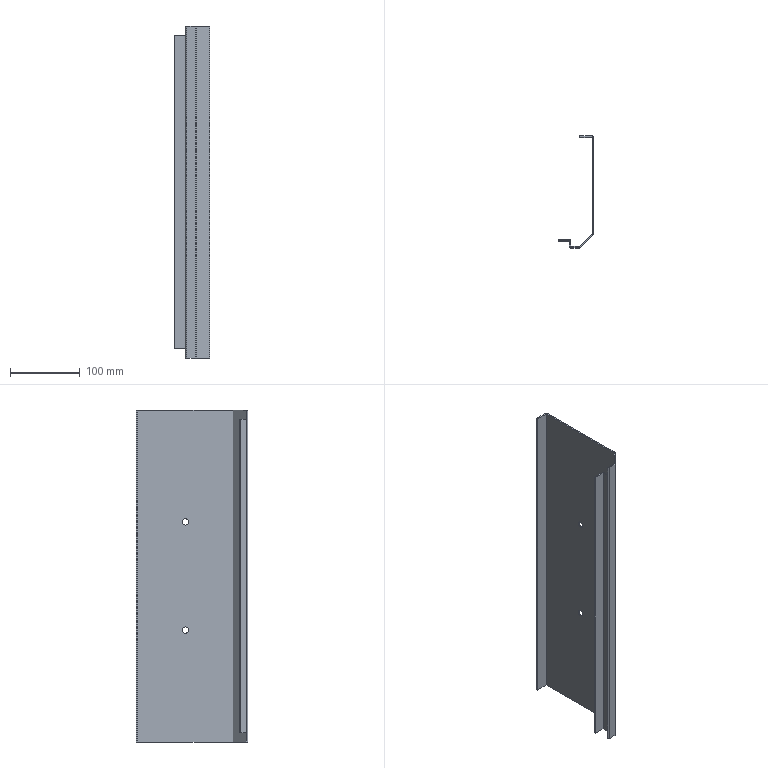Part | STEP file | Control Box 2 | 1 solid | 34 faces | box 51 x 160 x 476 mm | volume 211731 mm3 | plane 20 | cylinder 14 | commonest cylinder face diameters 0.2 x5 4.2 x5 9 x4
STEP:
#1=CARTESIAN_POINT('',(443.182,-70.615,320.));
#2=VERTEX_POINT('',#1);
#3=CARTESIAN_POINT('',(443.182,-70.615,311.));
#4=VERTEX_POINT('',#3);
#5=CARTESIAN_POINT('',(443.182,-70.615,315.5));
#6=DIRECTION('',(1.,0.,0.));
#7=DIRECTION('',(0.,0.,-1.));
#8=AXIS2_PLACEMENT_3D('',#5,#6,#7);
#9=CIRCLE('',#8,4.5);
#10=EDGE_CURVE('',#2,#4,#9,.T.);
#11=ORIENTED_EDGE('',*,*,#10,.F.);
#12=CARTESIAN_POINT('',(445.182,-70.615,320.));
#13=VERTEX_POINT('',#12);
#14=CARTESIAN_POINT('',(435.182,-70.615,320.));
#15=DIRECTION('',(1.,0.,0.));
#16=VECTOR('',#15,1000.);
#17=LINE('',#14,#16);
#18=EDGE_CURVE('',#2,#13,#17,.T.);
#19=ORIENTED_EDGE('',*,*,#18,.T.);
#20=CARTESIAN_POINT('',(445.182,-70.615,311.));
#21=VERTEX_POINT('',#20);
#22=CARTESIAN_POINT('',(445.182,-70.615,315.5));
#23=DIRECTION('',(-1.,0.,0.));
#24=DIRECTION('',(0.,0.,-1.));
#25=AXIS2_PLACEMENT_3D('',#22,#23,#24);
#26=CIRCLE('',#25,4.5);
#27=EDGE_CURVE('',#21,#13,#26,.T.);
#28=ORIENTED_EDGE('',*,*,#27,.F.);
#29=CARTESIAN_POINT('',(435.182,-70.615,311.));
#30=DIRECTION('',(1.,0.,0.));
#31=VECTOR('',#30,1000.);
#32=LINE('',#29,#31);
#33=EDGE_CURVE('',#4,#21,#32,.T.);
#34=ORIENTED_EDGE('',*,*,#33,.F.);
#35=EDGE_LOOP('',(#11,#19,#28,#34));
#36=FACE_OUTER_BOUND('',#35,.T.);
#37=CARTESIAN_POINT('',(435.182,-70.615,315.5));
#38=DIRECTION('',(1.,0.,0.));
#39=DIRECTION('',(0.,0.,-1.));
#40=AXIS2_PLACEMENT_3D('',#37,#38,#39);
#41=CYLINDRICAL_SURFACE('',#40,4.5);
#42=ADVANCED_FACE('',(#36),#41,.F.);
#43=CARTESIAN_POINT('',(443.182,-70.615,165.));
#44=VERTEX_POINT('',#43);
#45=CARTESIAN_POINT('',(443.182,-70.615,156.));
#46=VERTEX_POINT('',#45);
#47=CARTESIAN_POINT('',(443.182,-70.615,160.5));
#48=DIRECTION('',(1.,0.,0.));
#49=DIRECTION('',(0.,0.,-1.));
#50=AXIS2_PLACEMENT_3D('',#47,#48,#49);
#51=CIRCLE('',#50,4.5);
#52=EDGE_CURVE('',#44,#46,#51,.T.);
#53=ORIENTED_EDGE('',*,*,#52,.F.);
#54=CARTESIAN_POINT('',(445.182,-70.615,165.));
#55=VERTEX_POINT('',#54);
#56=CARTESIAN_POINT('',(435.182,-70.615,165.));
#57=DIRECTION('',(1.,0.,0.));
#58=VECTOR('',#57,1000.);
#59=LINE('',#56,#58);
#60=EDGE_CURVE('',#44,#55,#59,.T.);
#61=ORIENTED_EDGE('',*,*,#60,.T.);
#62=CARTESIAN_POINT('',(445.182,-70.615,156.));
#63=VERTEX_POINT('',#62);
#64=CARTESIAN_POINT('',(445.182,-70.615,160.5));
#65=DIRECTION('',(-1.,0.,0.));
#66=DIRECTION('',(0.,0.,-1.));
#67=AXIS2_PLACEMENT_3D('',#64,#65,#66);
#68=CIRCLE('',#67,4.5);
#69=EDGE_CURVE('',#63,#55,#68,.T.);
#70=ORIENTED_EDGE('',*,*,#69,.F.);
#71=CARTESIAN_POINT('',(435.182,-70.615,156.));
#72=DIRECTION('',(1.,0.,0.));
#73=VECTOR('',#72,1000.);
#74=LINE('',#71,#73);
#75=EDGE_CURVE('',#46,#63,#74,.T.);
#76=ORIENTED_EDGE('',*,*,#75,.F.);
#77=EDGE_LOOP('',(#53,#61,#70,#76));
#78=FACE_OUTER_BOUND('',#77,.T.);
#79=CARTESIAN_POINT('',(435.182,-70.615,160.5));
#80=DIRECTION('',(1.,0.,0.));
#81=DIRECTION('',(0.,0.,-1.));
#82=AXIS2_PLACEMENT_3D('',#79,#80,#81);
#83=CYLINDRICAL_SURFACE('',#82,4.5);
#84=ADVANCED_FACE('',(#78),#83,.F.);
#85=CARTESIAN_POINT('',(445.182,-2.1,476.));
#86=VERTEX_POINT('',#85);
#87=CARTESIAN_POINT('',(445.182,-139.13,476.));
#88=VERTEX_POINT('',#87);
#89=CARTESIAN_POINT('',(445.182,0.,476.));
#90=DIRECTION('',(0.,-1.,0.));
#91=VECTOR('',#90,1000.);
#92=LINE('',#89,#91);
#93=EDGE_CURVE('',#86,#88,#92,.T.);
#94=ORIENTED_EDGE('',*,*,#93,.T.);
#95=CARTESIAN_POINT('',(445.182,-139.13,0.));
#96=VERTEX_POINT('',#95);
#97=CARTESIAN_POINT('',(445.182,-139.13,476.));
#98=DIRECTION('',(0.,0.,-1.));
#99=VECTOR('',#98,1000.);
#100=LINE('',#97,#99);
#101=EDGE_CURVE('',#88,#96,#100,.T.);
#102=ORIENTED_EDGE('',*,*,#101,.T.);
#103=CARTESIAN_POINT('',(445.182,-2.1,0.));
#104=VERTEX_POINT('',#103);
#105=CARTESIAN_POINT('',(445.182,0.,0.));
#106=DIRECTION('',(0.,1.,0.));
#107=VECTOR('',#106,1000.);
#108=LINE('',#105,#107);
#109=EDGE_CURVE('',#96,#104,#108,.T.);
#110=ORIENTED_EDGE('',*,*,#109,.T.);
#111=CARTESIAN_POINT('',(445.182,-2.1,476.));
#112=DIRECTION('',(0.,0.,1.));
#113=VECTOR('',#112,1000.);
#114=LINE('',#111,#113);
#115=EDGE_CURVE('',#104,#86,#114,.T.);
#116=ORIENTED_EDGE('',*,*,#115,.T.);
#117=EDGE_LOOP('',(#94,#102,#110,#116));
#118=FACE_OUTER_BOUND('',#117,.T.);
#119=ORIENTED_EDGE('',*,*,#27,.T.);
#120=CARTESIAN_POINT('',(445.182,-70.615,315.5));
#121=DIRECTION('',(-1.,0.,0.));
#122=DIRECTION('',(0.,0.,-1.));
#123=AXIS2_PLACEMENT_3D('',#120,#121,#122);
#124=CIRCLE('',#123,4.5);
#125=EDGE_CURVE('',#13,#21,#124,.T.);
#126=ORIENTED_EDGE('',*,*,#125,.T.);
#127=EDGE_LOOP('',(#119,#126));
#128=FACE_BOUND('',#127,.T.);
#129=ORIENTED_EDGE('',*,*,#69,.T.);
#130=CARTESIAN_POINT('',(445.182,-70.615,160.5));
#131=DIRECTION('',(-1.,0.,0.));
#132=DIRECTION('',(0.,0.,-1.));
#133=AXIS2_PLACEMENT_3D('',#130,#131,#132);
#134=CIRCLE('',#133,4.5);
#135=EDGE_CURVE('',#55,#63,#134,.T.);
#136=ORIENTED_EDGE('',*,*,#135,.T.);
#137=EDGE_LOOP('',(#129,#136));
#138=FACE_BOUND('',#137,.T.);
#139=CARTESIAN_POINT('',(445.182,0.,476.));
#140=DIRECTION('',(1.,0.,0.));
#141=DIRECTION('',(0.,0.,-1.));
#142=AXIS2_PLACEMENT_3D('',#139,#140,#141);
#143=PLANE('',#142);
#144=ADVANCED_FACE('',(#118,#128,#138),#143,.T.);
#145=CARTESIAN_POINT('',(444.567,-140.615,476.));
#146=VERTEX_POINT('',#145);
#147=CARTESIAN_POINT('',(443.082,-139.13,476.));
#148=DIRECTION('',(0.,0.,1.));
#149=DIRECTION('',(-1.,0.,0.));
#150=AXIS2_PLACEMENT_3D('',#147,#148,#149);
#151=CIRCLE('',#150,2.1);
#152=EDGE_CURVE('',#146,#88,#151,.T.);
#153=ORIENTED_EDGE('',*,*,#152,.F.);
#154=CARTESIAN_POINT('',(444.567,-140.615,0.));
#155=VERTEX_POINT('',#154);
#156=CARTESIAN_POINT('',(444.567,-140.615,476.));
#157=DIRECTION('',(0.,0.,-1.));
#158=VECTOR('',#157,1000.);
#159=LINE('',#156,#158);
#160=EDGE_CURVE('',#146,#155,#159,.T.);
#161=ORIENTED_EDGE('',*,*,#160,.T.);
#162=CARTESIAN_POINT('',(443.082,-139.13,0.));
#163=DIRECTION('',(0.,0.,-1.));
#164=DIRECTION('',(-1.,0.,0.));
#165=AXIS2_PLACEMENT_3D('',#162,#163,#164);
#166=CIRCLE('',#165,2.1);
#167=EDGE_CURVE('',#96,#155,#166,.T.);
#168=ORIENTED_EDGE('',*,*,#167,.F.);
#169=ORIENTED_EDGE('',*,*,#101,.F.);
#170=EDGE_LOOP('',(#153,#161,#168,#169));
#171=FACE_OUTER_BOUND('',#170,.T.);
#172=CARTESIAN_POINT('',(443.082,-139.13,476.));
#173=DIRECTION('',(0.,0.,-1.));
#174=DIRECTION('',(-1.,0.,0.));
#175=AXIS2_PLACEMENT_3D('',#172,#173,#174);
#176=CYLINDRICAL_SURFACE('',#175,2.1);
#177=ADVANCED_FACE('',(#171),#176,.T.);
#178=CARTESIAN_POINT('',(443.182,-2.1,476.));
#179=VERTEX_POINT('',#178);
#180=CARTESIAN_POINT('',(443.182,-139.13,476.));
#181=VERTEX_POINT('',#180);
#182=CARTESIAN_POINT('',(443.182,-2.,476.));
#183=DIRECTION('',(0.,-1.,0.));
#184=VECTOR('',#183,1000.);
#185=LINE('',#182,#184);
#186=EDGE_CURVE('',#179,#181,#185,.T.);
#187=ORIENTED_EDGE('',*,*,#186,.T.);
#188=CARTESIAN_POINT('',(443.153,-139.201,476.));
#189=VERTEX_POINT('',#188);
#190=CARTESIAN_POINT('',(443.082,-139.13,476.));
#191=DIRECTION('',(0.,0.,-1.));
#192=DIRECTION('',(-1.,0.,0.));
#193=AXIS2_PLACEMENT_3D('',#190,#191,#192);
#194=CIRCLE('',#193,0.1);
#195=EDGE_CURVE('',#181,#189,#194,.T.);
#196=ORIENTED_EDGE('',*,*,#195,.T.);
#197=CARTESIAN_POINT('',(424.383,-157.971,476.));
#198=VERTEX_POINT('',#197);
#199=CARTESIAN_POINT('',(443.153,-139.201,476.));
#200=DIRECTION('',(-0.7071,-0.7071,0.));
#201=VECTOR('',#200,1000.);
#202=LINE('',#199,#201);
#203=EDGE_CURVE('',#189,#198,#202,.T.);
#204=ORIENTED_EDGE('',*,*,#203,.T.);
#205=CARTESIAN_POINT('',(424.312,-158.,476.));
#206=VERTEX_POINT('',#205);
#207=CARTESIAN_POINT('',(424.312,-157.9,476.));
#208=DIRECTION('',(0.,0.,-1.));
#209=DIRECTION('',(-1.,0.,0.));
#210=AXIS2_PLACEMENT_3D('',#207,#208,#209);
#211=CIRCLE('',#210,0.1);
#212=EDGE_CURVE('',#198,#206,#211,.T.);
#213=ORIENTED_EDGE('',*,*,#212,.T.);
#214=CARTESIAN_POINT('',(412.282,-158.,476.));
#215=VERTEX_POINT('',#214);
#216=CARTESIAN_POINT('',(424.383,-158.,476.));
#217=DIRECTION('',(-1.,0.,0.));
#218=VECTOR('',#217,1000.);
#219=LINE('',#216,#218);
#220=EDGE_CURVE('',#206,#215,#219,.T.);
#221=ORIENTED_EDGE('',*,*,#220,.T.);
#222=CARTESIAN_POINT('',(412.182,-157.9,476.));
#223=VERTEX_POINT('',#222);
#224=CARTESIAN_POINT('',(412.282,-157.9,476.));
#225=DIRECTION('',(0.,0.,-1.));
#226=DIRECTION('',(-1.,0.,0.));
#227=AXIS2_PLACEMENT_3D('',#224,#225,#226);
#228=CIRCLE('',#227,0.1);
#229=EDGE_CURVE('',#215,#223,#228,.T.);
#230=ORIENTED_EDGE('',*,*,#229,.T.);
#231=CARTESIAN_POINT('',(410.182,-157.9,476.));
#232=VERTEX_POINT('',#231);
#233=CARTESIAN_POINT('',(412.182,-157.9,476.));
#234=DIRECTION('',(1.,0.,0.));
#235=VECTOR('',#234,1000.);
#236=LINE('',#233,#235);
#237=EDGE_CURVE('',#232,#223,#236,.T.);
#238=ORIENTED_EDGE('',*,*,#237,.F.);
#239=CARTESIAN_POINT('',(412.282,-160.,476.));
#240=VERTEX_POINT('',#239);
#241=CARTESIAN_POINT('',(412.282,-157.9,476.));
#242=DIRECTION('',(0.,0.,-1.));
#243=DIRECTION('',(-1.,0.,0.));
#244=AXIS2_PLACEMENT_3D('',#241,#242,#243);
#245=CIRCLE('',#244,2.1);
#246=EDGE_CURVE('',#240,#232,#245,.T.);
#247=ORIENTED_EDGE('',*,*,#246,.F.);
#248=CARTESIAN_POINT('',(424.312,-160.,476.));
#249=VERTEX_POINT('',#248);
#250=CARTESIAN_POINT('',(425.182,-160.,476.));
#251=DIRECTION('',(-1.,0.,0.));
#252=VECTOR('',#251,1000.);
#253=LINE('',#250,#252);
#254=EDGE_CURVE('',#249,#240,#253,.T.);
#255=ORIENTED_EDGE('',*,*,#254,.F.);
#256=CARTESIAN_POINT('',(425.797,-159.385,476.));
#257=VERTEX_POINT('',#256);
#258=CARTESIAN_POINT('',(424.312,-157.9,476.));
#259=DIRECTION('',(0.,0.,1.));
#260=DIRECTION('',(-1.,0.,0.));
#261=AXIS2_PLACEMENT_3D('',#258,#259,#260);
#262=CIRCLE('',#261,2.1);
#263=EDGE_CURVE('',#249,#257,#262,.T.);
#264=ORIENTED_EDGE('',*,*,#263,.T.);
#265=CARTESIAN_POINT('',(425.182,-160.,476.));
#266=DIRECTION('',(-0.7071,-0.7071,0.));
#267=VECTOR('',#266,1000.);
#268=LINE('',#265,#267);
#269=EDGE_CURVE('',#146,#257,#268,.T.);
#270=ORIENTED_EDGE('',*,*,#269,.F.);
#271=ORIENTED_EDGE('',*,*,#152,.T.);
#272=ORIENTED_EDGE('',*,*,#93,.F.);
#273=CARTESIAN_POINT('',(443.082,0.,476.));
#274=VERTEX_POINT('',#273);
#275=CARTESIAN_POINT('',(443.082,-2.1,476.));
#276=DIRECTION('',(0.,0.,-1.));
#277=DIRECTION('',(-1.,0.,0.));
#278=AXIS2_PLACEMENT_3D('',#275,#276,#277);
#279=CIRCLE('',#278,2.1);
#280=EDGE_CURVE('',#274,#86,#279,.T.);
#281=ORIENTED_EDGE('',*,*,#280,.F.);
#282=CARTESIAN_POINT('',(425.182,0.,476.));
#283=VERTEX_POINT('',#282);
#284=CARTESIAN_POINT('',(425.182,0.,476.));
#285=DIRECTION('',(1.,0.,0.));
#286=VECTOR('',#285,1000.);
#287=LINE('',#284,#286);
#288=EDGE_CURVE('',#283,#274,#287,.T.);
#289=ORIENTED_EDGE('',*,*,#288,.F.);
#290=CARTESIAN_POINT('',(425.182,-2.,476.));
#291=VERTEX_POINT('',#290);
#292=CARTESIAN_POINT('',(425.182,-150.1,476.));
#293=DIRECTION('',(0.,1.,0.));
#294=VECTOR('',#293,1000.);
#295=LINE('',#292,#294);
#296=EDGE_CURVE('',#291,#283,#295,.T.);
#297=ORIENTED_EDGE('',*,*,#296,.F.);
#298=CARTESIAN_POINT('',(443.082,-2.,476.));
#299=VERTEX_POINT('',#298);
#300=CARTESIAN_POINT('',(410.082,-2.,476.));
#301=DIRECTION('',(-1.,0.,0.));
#302=VECTOR('',#301,1000.);
#303=LINE('',#300,#302);
#304=EDGE_CURVE('',#299,#291,#303,.T.);
#305=ORIENTED_EDGE('',*,*,#304,.F.);
#306=CARTESIAN_POINT('',(443.082,-2.1,476.));
#307=DIRECTION('',(0.,0.,-1.));
#308=DIRECTION('',(-1.,0.,0.));
#309=AXIS2_PLACEMENT_3D('',#306,#307,#308);
#310=CIRCLE('',#309,0.1);
#311=EDGE_CURVE('',#299,#179,#310,.T.);
#312=ORIENTED_EDGE('',*,*,#311,.T.);
#313=EDGE_LOOP('',(#187,#196,#204,#213,#221,#230,#238,#247,#255,#264,#270,#271,#272,#281,#289,#297,#305,#312));
#314=FACE_OUTER_BOUND('',#313,.T.);
#315=CARTESIAN_POINT('',(443.082,-2.,476.));
#316=DIRECTION('',(0.,0.,1.));
#317=DIRECTION('',(1.,0.,0.));
#318=AXIS2_PLACEMENT_3D('',#315,#316,#317);
#319=PLANE('',#318);
#320=ADVANCED_FACE('',(#314),#319,.T.);
#321=ORIENTED_EDGE('',*,*,#280,.T.);
#322=ORIENTED_EDGE('',*,*,#115,.F.);
#323=CARTESIAN_POINT('',(443.082,0.,0.));
#324=VERTEX_POINT('',#323);
#325=CARTESIAN_POINT('',(443.082,-2.1,0.));
#326=DIRECTION('',(0.,0.,1.));
#327=DIRECTION('',(-1.,0.,0.));
#328=AXIS2_PLACEMENT_3D('',#325,#326,#327);
#329=CIRCLE('',#328,2.1);
#330=EDGE_CURVE('',#104,#324,#329,.T.);
#331=ORIENTED_EDGE('',*,*,#330,.T.);
#332=CARTESIAN_POINT('',(443.082,0.,476.));
#333=DIRECTION('',(0.,0.,1.));
#334=VECTOR('',#333,1000.);
#335=LINE('',#332,#334);
#336=EDGE_CURVE('',#324,#274,#335,.T.);
#337=ORIENTED_EDGE('',*,*,#336,.T.);
#338=EDGE_LOOP('',(#321,#322,#331,#337));
#339=FACE_OUTER_BOUND('',#338,.T.);
#340=CARTESIAN_POINT('',(443.082,-2.1,476.));
#341=DIRECTION('',(0.,0.,-1.));
#342=DIRECTION('',(-1.,0.,0.));
#343=AXIS2_PLACEMENT_3D('',#340,#341,#342);
#344=CYLINDRICAL_SURFACE('',#343,2.1);
#345=ADVANCED_FACE('',(#339),#344,.T.);
#346=CARTESIAN_POINT('',(443.182,-139.13,0.));
#347=VERTEX_POINT('',#346);
#348=CARTESIAN_POINT('',(443.182,-2.1,0.));
#349=VERTEX_POINT('',#348);
#350=CARTESIAN_POINT('',(443.182,-139.201,0.));
#351=DIRECTION('',(0.,1.,0.));
#352=VECTOR('',#351,1000.);
#353=LINE('',#350,#352);
#354=EDGE_CURVE('',#347,#349,#353,.T.);
#355=ORIENTED_EDGE('',*,*,#354,.T.);
#356=CARTESIAN_POINT('',(443.082,-2.,0.));
#357=VERTEX_POINT('',#356);
#358=CARTESIAN_POINT('',(443.082,-2.1,0.));
#359=DIRECTION('',(0.,0.,1.));
#360=DIRECTION('',(-1.,0.,0.));
#361=AXIS2_PLACEMENT_3D('',#358,#359,#360);
#362=CIRCLE('',#361,0.1);
#363=EDGE_CURVE('',#349,#357,#362,.T.);
#364=ORIENTED_EDGE('',*,*,#363,.T.);
#365=CARTESIAN_POINT('',(425.182,-2.,0.));
#366=VERTEX_POINT('',#365);
#367=CARTESIAN_POINT('',(443.182,-2.,0.));
#368=DIRECTION('',(-1.,0.,0.));
#369=VECTOR('',#368,1000.);
#370=LINE('',#367,#369);
#371=EDGE_CURVE('',#357,#366,#370,.T.);
#372=ORIENTED_EDGE('',*,*,#371,.T.);
#373=CARTESIAN_POINT('',(425.182,0.,0.));
#374=VERTEX_POINT('',#373);
#375=CARTESIAN_POINT('',(425.182,-2.,0.));
#376=DIRECTION('',(0.,-1.,0.));
#377=VECTOR('',#376,1000.);
#378=LINE('',#375,#377);
#379=EDGE_CURVE('',#374,#366,#378,.T.);
#380=ORIENTED_EDGE('',*,*,#379,.F.);
#381=CARTESIAN_POINT('',(425.182,0.,0.));
#382=DIRECTION('',(-1.,0.,0.));
#383=VECTOR('',#382,1000.);
#384=LINE('',#381,#383);
#385=EDGE_CURVE('',#324,#374,#384,.T.);
#386=ORIENTED_EDGE('',*,*,#385,.F.);
#387=ORIENTED_EDGE('',*,*,#330,.F.);
#388=ORIENTED_EDGE('',*,*,#109,.F.);
#389=ORIENTED_EDGE('',*,*,#167,.T.);
#390=CARTESIAN_POINT('',(425.797,-159.385,0.));
#391=VERTEX_POINT('',#390);
#392=CARTESIAN_POINT('',(425.182,-160.,0.));
#393=DIRECTION('',(0.7071,0.7071,0.));
#394=VECTOR('',#393,1000.);
#395=LINE('',#392,#394);
#396=EDGE_CURVE('',#391,#155,#395,.T.);
#397=ORIENTED_EDGE('',*,*,#396,.F.);
#398=CARTESIAN_POINT('',(424.312,-160.,0.));
#399=VERTEX_POINT('',#398);
#400=CARTESIAN_POINT('',(424.312,-157.9,0.));
#401=DIRECTION('',(0.,0.,-1.));
#402=DIRECTION('',(-1.,0.,0.));
#403=AXIS2_PLACEMENT_3D('',#400,#401,#402);
#404=CIRCLE('',#403,2.1);
#405=EDGE_CURVE('',#391,#399,#404,.T.);
#406=ORIENTED_EDGE('',*,*,#405,.T.);
#407=CARTESIAN_POINT('',(412.282,-160.,0.));
#408=VERTEX_POINT('',#407);
#409=CARTESIAN_POINT('',(425.182,-160.,0.));
#410=DIRECTION('',(1.,0.,0.));
#411=VECTOR('',#410,1000.);
#412=LINE('',#409,#411);
#413=EDGE_CURVE('',#408,#399,#412,.T.);
#414=ORIENTED_EDGE('',*,*,#413,.F.);
#415=CARTESIAN_POINT('',(410.182,-157.9,0.));
#416=VERTEX_POINT('',#415);
#417=CARTESIAN_POINT('',(412.282,-157.9,0.));
#418=DIRECTION('',(0.,0.,1.));
#419=DIRECTION('',(-1.,0.,0.));
#420=AXIS2_PLACEMENT_3D('',#417,#418,#419);
#421=CIRCLE('',#420,2.1);
#422=EDGE_CURVE('',#416,#408,#421,.T.);
#423=ORIENTED_EDGE('',*,*,#422,.F.);
#424=CARTESIAN_POINT('',(412.182,-157.9,0.));
#425=VERTEX_POINT('',#424);
#426=CARTESIAN_POINT('',(412.182,-157.9,0.));
#427=DIRECTION('',(1.,0.,0.));
#428=VECTOR('',#427,1000.);
#429=LINE('',#426,#428);
#430=EDGE_CURVE('',#416,#425,#429,.T.);
#431=ORIENTED_EDGE('',*,*,#430,.T.);
#432=CARTESIAN_POINT('',(412.282,-158.,0.));
#433=VERTEX_POINT('',#432);
#434=CARTESIAN_POINT('',(412.282,-157.9,0.));
#435=DIRECTION('',(0.,0.,1.));
#436=DIRECTION('',(-1.,0.,0.));
#437=AXIS2_PLACEMENT_3D('',#434,#435,#436);
#438=CIRCLE('',#437,0.1);
#439=EDGE_CURVE('',#425,#433,#438,.T.);
#440=ORIENTED_EDGE('',*,*,#439,.T.);
#441=CARTESIAN_POINT('',(424.312,-158.,0.));
#442=VERTEX_POINT('',#441);
#443=CARTESIAN_POINT('',(412.182,-158.,0.));
#444=DIRECTION('',(1.,0.,0.));
#445=VECTOR('',#444,1000.);
#446=LINE('',#443,#445);
#447=EDGE_CURVE('',#433,#442,#446,.T.);
#448=ORIENTED_EDGE('',*,*,#447,.T.);
#449=CARTESIAN_POINT('',(424.383,-157.971,0.));
#450=VERTEX_POINT('',#449);
#451=CARTESIAN_POINT('',(424.312,-157.9,0.));
#452=DIRECTION('',(0.,0.,1.));
#453=DIRECTION('',(-1.,0.,0.));
#454=AXIS2_PLACEMENT_3D('',#451,#452,#453);
#455=CIRCLE('',#454,0.1);
#456=EDGE_CURVE('',#442,#450,#455,.T.);
#457=ORIENTED_EDGE('',*,*,#456,.T.);
#458=CARTESIAN_POINT('',(443.153,-139.201,0.));
#459=VERTEX_POINT('',#458);
#460=CARTESIAN_POINT('',(424.383,-157.971,0.));
#461=DIRECTION('',(0.7071,0.7071,0.));
#462=VECTOR('',#461,1000.);
#463=LINE('',#460,#462);
#464=EDGE_CURVE('',#450,#459,#463,.T.);
#465=ORIENTED_EDGE('',*,*,#464,.T.);
#466=CARTESIAN_POINT('',(443.082,-139.13,0.));
#467=DIRECTION('',(0.,0.,1.));
#468=DIRECTION('',(-1.,0.,0.));
#469=AXIS2_PLACEMENT_3D('',#466,#467,#468);
#470=CIRCLE('',#469,0.1);
#471=EDGE_CURVE('',#459,#347,#470,.T.);
#472=ORIENTED_EDGE('',*,*,#471,.T.);
#473=EDGE_LOOP('',(#355,#364,#372,#380,#386,#387,#388,#389,#397,#406,#414,#423,#431,#440,#448,#457,#465,#472));
#474=FACE_OUTER_BOUND('',#473,.T.);
#475=CARTESIAN_POINT('',(443.153,-139.201,0.));
#476=DIRECTION('',(0.,0.,-1.));
#477=DIRECTION('',(-1.,0.,0.));
#478=AXIS2_PLACEMENT_3D('',#475,#476,#477);
#479=PLANE('',#478);
#480=ADVANCED_FACE('',(#474),#479,.T.);
#481=ORIENTED_EDGE('',*,*,#18,.F.);
#482=CARTESIAN_POINT('',(443.182,-70.615,315.5));
#483=DIRECTION('',(1.,0.,0.));
#484=DIRECTION('',(0.,0.,-1.));
#485=AXIS2_PLACEMENT_3D('',#482,#483,#484);
#486=CIRCLE('',#485,4.5);
#487=EDGE_CURVE('',#4,#2,#486,.T.);
#488=ORIENTED_EDGE('',*,*,#487,.F.);
#489=ORIENTED_EDGE('',*,*,#33,.T.);
#490=ORIENTED_EDGE('',*,*,#125,.F.);
#491=EDGE_LOOP('',(#481,#488,#489,#490));
#492=FACE_OUTER_BOUND('',#491,.T.);
#493=CARTESIAN_POINT('',(435.182,-70.615,315.5));
#494=DIRECTION('',(1.,0.,0.));
#495=DIRECTION('',(0.,0.,-1.));
#496=AXIS2_PLACEMENT_3D('',#493,#494,#495);
#497=CYLINDRICAL_SURFACE('',#496,4.5);
#498=ADVANCED_FACE('',(#492),#497,.F.);
#499=ORIENTED_EDGE('',*,*,#60,.F.);
#500=CARTESIAN_POINT('',(443.182,-70.615,160.5));
#501=DIRECTION('',(1.,0.,0.));
#502=DIRECTION('',(0.,0.,-1.));
#503=AXIS2_PLACEMENT_3D('',#500,#501,#502);
#504=CIRCLE('',#503,4.5);
#505=EDGE_CURVE('',#46,#44,#504,.T.);
#506=ORIENTED_EDGE('',*,*,#505,.F.);
#507=ORIENTED_EDGE('',*,*,#75,.T.);
#508=ORIENTED_EDGE('',*,*,#135,.F.);
#509=EDGE_LOOP('',(#499,#506,#507,#508));
#510=FACE_OUTER_BOUND('',#509,.T.);
#511=CARTESIAN_POINT('',(435.182,-70.615,160.5));
#512=DIRECTION('',(1.,0.,0.));
#513=DIRECTION('',(0.,0.,-1.));
#514=AXIS2_PLACEMENT_3D('',#511,#512,#513);
#515=CYLINDRICAL_SURFACE('',#514,4.5);
#516=ADVANCED_FACE('',(#510),#515,.F.);
#517=ORIENTED_EDGE('',*,*,#269,.T.);
#518=CARTESIAN_POINT('',(425.797,-159.385,476.));
#519=DIRECTION('',(0.,0.,-1.));
#520=VECTOR('',#519,1000.);
#521=LINE('',#518,#520);
#522=EDGE_CURVE('',#257,#391,#521,.T.);
#523=ORIENTED_EDGE('',*,*,#522,.T.);
#524=ORIENTED_EDGE('',*,*,#396,.T.);
#525=ORIENTED_EDGE('',*,*,#160,.F.);
#526=EDGE_LOOP('',(#517,#523,#524,#525));
#527=FACE_OUTER_BOUND('',#526,.T.);
#528=CARTESIAN_POINT('',(425.182,-160.,476.));
#529=DIRECTION('',(0.7071,-0.7071,0.));
#530=DIRECTION('',(0.7071,0.7071,0.));
#531=AXIS2_PLACEMENT_3D('',#528,#529,#530);
#532=PLANE('',#531);
#533=ADVANCED_FACE('',(#527),#532,.T.);
#534=CARTESIAN_POINT('',(443.182,-139.13,476.));
#535=DIRECTION('',(0.,0.,-1.));
#536=VECTOR('',#535,1000.);
#537=LINE('',#534,#536);
#538=EDGE_CURVE('',#181,#347,#537,.T.);
#539=ORIENTED_EDGE('',*,*,#538,.F.);
#540=ORIENTED_EDGE('',*,*,#186,.F.);
#541=CARTESIAN_POINT('',(443.182,-2.1,476.));
#542=DIRECTION('',(0.,0.,1.));
#543=VECTOR('',#542,1000.);
#544=LINE('',#541,#543);
#545=EDGE_CURVE('',#349,#179,#544,.T.);
#546=ORIENTED_EDGE('',*,*,#545,.F.);
#547=ORIENTED_EDGE('',*,*,#354,.F.);
#548=EDGE_LOOP('',(#539,#540,#546,#547));
#549=FACE_OUTER_BOUND('',#548,.T.);
#550=ORIENTED_EDGE('',*,*,#487,.T.);
#551=ORIENTED_EDGE('',*,*,#10,.T.);
#552=EDGE_LOOP('',(#550,#551));
#553=FACE_BOUND('',#552,.T.);
#554=ORIENTED_EDGE('',*,*,#505,.T.);
#555=ORIENTED_EDGE('',*,*,#52,.T.);
#556=EDGE_LOOP('',(#554,#555));
#557=FACE_BOUND('',#556,.T.);
#558=CARTESIAN_POINT('',(443.182,0.,476.));
#559=DIRECTION('',(1.,0.,0.));
#560=DIRECTION('',(0.,0.,-1.));
#561=AXIS2_PLACEMENT_3D('',#558,#559,#560);
#562=PLANE('',#561);
#563=ADVANCED_FACE('',(#549,#553,#557),#562,.F.);
#564=ORIENTED_EDGE('',*,*,#288,.T.);
#565=ORIENTED_EDGE('',*,*,#336,.F.);
#566=ORIENTED_EDGE('',*,*,#385,.T.);
#567=CARTESIAN_POINT('',(425.182,0.,476.));
#568=DIRECTION('',(0.,0.,1.));
#569=VECTOR('',#568,1000.);
#570=LINE('',#567,#569);
#571=EDGE_CURVE('',#374,#283,#570,.T.);
#572=ORIENTED_EDGE('',*,*,#571,.T.);
#573=EDGE_LOOP('',(#564,#565,#566,#572));
#574=FACE_OUTER_BOUND('',#573,.T.);
#575=CARTESIAN_POINT('',(425.182,0.,476.));
#576=DIRECTION('',(0.,1.,0.));
#577=DIRECTION('',(0.,0.,1.));
#578=AXIS2_PLACEMENT_3D('',#575,#576,#577);
#579=PLANE('',#578);
#580=ADVANCED_FACE('',(#574),#579,.T.);
#581=ORIENTED_EDGE('',*,*,#263,.F.);
#582=CARTESIAN_POINT('',(424.312,-160.,476.));
#583=DIRECTION('',(0.,0.,-1.));
#584=VECTOR('',#583,1000.);
#585=LINE('',#582,#584);
#586=EDGE_CURVE('',#249,#399,#585,.T.);
#587=ORIENTED_EDGE('',*,*,#586,.T.);
#588=ORIENTED_EDGE('',*,*,#405,.F.);
#589=ORIENTED_EDGE('',*,*,#522,.F.);
#590=EDGE_LOOP('',(#581,#587,#588,#589));
#591=FACE_OUTER_BOUND('',#590,.T.);
#592=CARTESIAN_POINT('',(424.312,-157.9,476.));
#593=DIRECTION('',(0.,0.,-1.));
#594=DIRECTION('',(-1.,0.,0.));
#595=AXIS2_PLACEMENT_3D('',#592,#593,#594);
#596=CYLINDRICAL_SURFACE('',#595,2.1);
#597=ADVANCED_FACE('',(#591),#596,.T.);
#598=CARTESIAN_POINT('',(443.153,-139.201,476.));
#599=DIRECTION('',(0.,0.,-1.));
#600=VECTOR('',#599,1000.);
#601=LINE('',#598,#600);
#602=EDGE_CURVE('',#189,#459,#601,.T.);
#603=ORIENTED_EDGE('',*,*,#602,.F.);
#604=ORIENTED_EDGE('',*,*,#195,.F.);
#605=ORIENTED_EDGE('',*,*,#538,.T.);
#606=ORIENTED_EDGE('',*,*,#471,.F.);
#607=EDGE_LOOP('',(#603,#604,#605,#606));
#608=FACE_OUTER_BOUND('',#607,.T.);
#609=CARTESIAN_POINT('',(443.082,-139.13,476.));
#610=DIRECTION('',(0.,0.,-1.));
#611=DIRECTION('',(-1.,0.,0.));
#612=AXIS2_PLACEMENT_3D('',#609,#610,#611);
#613=CYLINDRICAL_SURFACE('',#612,0.1);
#614=ADVANCED_FACE('',(#608),#613,.F.);
#615=ORIENTED_EDGE('',*,*,#545,.T.);
#616=ORIENTED_EDGE('',*,*,#311,.F.);
#617=CARTESIAN_POINT('',(443.082,-2.,476.));
#618=DIRECTION('',(0.,0.,1.));
#619=VECTOR('',#618,1000.);
#620=LINE('',#617,#619);
#621=EDGE_CURVE('',#357,#299,#620,.T.);
#622=ORIENTED_EDGE('',*,*,#621,.F.);
#623=ORIENTED_EDGE('',*,*,#363,.F.);
#624=EDGE_LOOP('',(#615,#616,#622,#623));
#625=FACE_OUTER_BOUND('',#624,.T.);
#626=CARTESIAN_POINT('',(443.082,-2.1,476.));
#627=DIRECTION('',(0.,0.,-1.));
#628=DIRECTION('',(-1.,0.,0.));
#629=AXIS2_PLACEMENT_3D('',#626,#627,#628);
#630=CYLINDRICAL_SURFACE('',#629,0.1);
#631=ADVANCED_FACE('',(#625),#630,.F.);
#632=ORIENTED_EDGE('',*,*,#296,.T.);
#633=ORIENTED_EDGE('',*,*,#571,.F.);
#634=ORIENTED_EDGE('',*,*,#379,.T.);
#635=CARTESIAN_POINT('',(425.182,-2.,476.));
#636=DIRECTION('',(0.,0.,1.));
#637=VECTOR('',#636,1000.);
#638=LINE('',#635,#637);
#639=EDGE_CURVE('',#366,#291,#638,.T.);
#640=ORIENTED_EDGE('',*,*,#639,.T.);
#641=EDGE_LOOP('',(#632,#633,#634,#640));
#642=FACE_OUTER_BOUND('',#641,.T.);
#643=CARTESIAN_POINT('',(425.182,-2.,476.));
#644=DIRECTION('',(-1.,0.,0.));
#645=DIRECTION('',(0.,0.,1.));
#646=AXIS2_PLACEMENT_3D('',#643,#644,#645);
#647=PLANE('',#646);
#648=ADVANCED_FACE('',(#642),#647,.T.);
#649=ORIENTED_EDGE('',*,*,#254,.T.);
#650=CARTESIAN_POINT('',(412.282,-160.,476.));
#651=DIRECTION('',(0.,0.,-1.));
#652=VECTOR('',#651,1000.);
#653=LINE('',#650,#652);
#654=EDGE_CURVE('',#240,#408,#653,.T.);
#655=ORIENTED_EDGE('',*,*,#654,.T.);
#656=ORIENTED_EDGE('',*,*,#413,.T.);
#657=ORIENTED_EDGE('',*,*,#586,.F.);
#658=EDGE_LOOP('',(#649,#655,#656,#657));
#659=FACE_OUTER_BOUND('',#658,.T.);
#660=CARTESIAN_POINT('',(425.182,-160.,476.));
#661=DIRECTION('',(0.,-1.,0.));
#662=DIRECTION('',(0.,0.,-1.));
#663=AXIS2_PLACEMENT_3D('',#660,#661,#662);
#664=PLANE('',#663);
#665=ADVANCED_FACE('',(#659),#664,.T.);
#666=CARTESIAN_POINT('',(424.383,-157.971,476.));
#667=DIRECTION('',(0.,0.,-1.));
#668=VECTOR('',#667,1000.);
#669=LINE('',#666,#668);
#670=EDGE_CURVE('',#198,#450,#669,.T.);
#671=ORIENTED_EDGE('',*,*,#670,.F.);
#672=ORIENTED_EDGE('',*,*,#203,.F.);
#673=ORIENTED_EDGE('',*,*,#602,.T.);
#674=ORIENTED_EDGE('',*,*,#464,.F.);
#675=EDGE_LOOP('',(#671,#672,#673,#674));
#676=FACE_OUTER_BOUND('',#675,.T.);
#677=CARTESIAN_POINT('',(423.768,-158.586,476.));
#678=DIRECTION('',(0.7071,-0.7071,0.));
#679=DIRECTION('',(0.7071,0.7071,0.));
#680=AXIS2_PLACEMENT_3D('',#677,#678,#679);
#681=PLANE('',#680);
#682=ADVANCED_FACE('',(#676),#681,.F.);
#683=ORIENTED_EDGE('',*,*,#621,.T.);
#684=ORIENTED_EDGE('',*,*,#304,.T.);
#685=ORIENTED_EDGE('',*,*,#639,.F.);
#686=ORIENTED_EDGE('',*,*,#371,.F.);
#687=EDGE_LOOP('',(#683,#684,#685,#686));
#688=FACE_OUTER_BOUND('',#687,.T.);
#689=CARTESIAN_POINT('',(425.182,-2.,476.));
#690=DIRECTION('',(0.,1.,0.));
#691=DIRECTION('',(0.,0.,1.));
#692=AXIS2_PLACEMENT_3D('',#689,#690,#691);
#693=PLANE('',#692);
#694=ADVANCED_FACE('',(#688),#693,.F.);
#695=CARTESIAN_POINT('',(410.182,-157.9,462.5));
#696=VERTEX_POINT('',#695);
#697=CARTESIAN_POINT('',(410.182,-157.9,13.5));
#698=VERTEX_POINT('',#697);
#699=CARTESIAN_POINT('',(410.182,-157.9,476.));
#700=DIRECTION('',(0.,0.,-1.));
#701=VECTOR('',#700,1000.);
#702=LINE('',#699,#701);
#703=EDGE_CURVE('',#696,#698,#702,.T.);
#704=ORIENTED_EDGE('',*,*,#703,.T.);
#705=CARTESIAN_POINT('',(410.182,-157.9,476.));
#706=DIRECTION('',(0.,0.,-1.));
#707=VECTOR('',#706,1000.);
#708=LINE('',#705,#707);
#709=EDGE_CURVE('',#698,#416,#708,.T.);
#710=ORIENTED_EDGE('',*,*,#709,.T.);
#711=ORIENTED_EDGE('',*,*,#422,.T.);
#712=ORIENTED_EDGE('',*,*,#654,.F.);
#713=ORIENTED_EDGE('',*,*,#246,.T.);
#714=CARTESIAN_POINT('',(410.182,-157.9,476.));
#715=DIRECTION('',(0.,0.,-1.));
#716=VECTOR('',#715,1000.);
#717=LINE('',#714,#716);
#718=EDGE_CURVE('',#232,#696,#717,.T.);
#719=ORIENTED_EDGE('',*,*,#718,.T.);
#720=EDGE_LOOP('',(#704,#710,#711,#712,#713,#719));
#721=FACE_OUTER_BOUND('',#720,.T.);
#722=CARTESIAN_POINT('',(412.282,-157.9,476.));
#723=DIRECTION('',(0.,0.,-1.));
#724=DIRECTION('',(-1.,0.,0.));
#725=AXIS2_PLACEMENT_3D('',#722,#723,#724);
#726=CYLINDRICAL_SURFACE('',#725,2.1);
#727=ADVANCED_FACE('',(#721),#726,.T.);
#728=CARTESIAN_POINT('',(424.312,-158.,476.));
#729=DIRECTION('',(0.,0.,-1.));
#730=VECTOR('',#729,1000.);
#731=LINE('',#728,#730);
#732=EDGE_CURVE('',#206,#442,#731,.T.);
#733=ORIENTED_EDGE('',*,*,#732,.F.);
#734=ORIENTED_EDGE('',*,*,#212,.F.);
#735=ORIENTED_EDGE('',*,*,#670,.T.);
#736=ORIENTED_EDGE('',*,*,#456,.F.);
#737=EDGE_LOOP('',(#733,#734,#735,#736));
#738=FACE_OUTER_BOUND('',#737,.T.);
#739=CARTESIAN_POINT('',(424.312,-157.9,476.));
#740=DIRECTION('',(0.,0.,-1.));
#741=DIRECTION('',(-1.,0.,0.));
#742=AXIS2_PLACEMENT_3D('',#739,#740,#741);
#743=CYLINDRICAL_SURFACE('',#742,0.1);
#744=ADVANCED_FACE('',(#738),#743,.F.);
#745=ORIENTED_EDGE('',*,*,#430,.F.);
#746=ORIENTED_EDGE('',*,*,#709,.F.);
#747=CARTESIAN_POINT('',(412.182,-157.9,13.5));
#748=VERTEX_POINT('',#747);
#749=CARTESIAN_POINT('',(412.182,-157.9,13.5));
#750=DIRECTION('',(-1.,0.,0.));
#751=VECTOR('',#750,1000.);
#752=LINE('',#749,#751);
#753=EDGE_CURVE('',#748,#698,#752,.T.);
#754=ORIENTED_EDGE('',*,*,#753,.F.);
#755=CARTESIAN_POINT('',(412.182,-157.9,0.));
#756=DIRECTION('',(0.,0.,1.));
#757=VECTOR('',#756,1000.);
#758=LINE('',#755,#757);
#759=EDGE_CURVE('',#425,#748,#758,.T.);
#760=ORIENTED_EDGE('',*,*,#759,.F.);
#761=EDGE_LOOP('',(#745,#746,#754,#760));
#762=FACE_OUTER_BOUND('',#761,.T.);
#763=CARTESIAN_POINT('',(412.182,-157.9,0.));
#764=DIRECTION('',(0.,-1.,0.));
#765=DIRECTION('',(0.,0.,-1.));
#766=AXIS2_PLACEMENT_3D('',#763,#764,#765);
#767=PLANE('',#766);
#768=ADVANCED_FACE('',(#762),#767,.F.);
#769=ORIENTED_EDGE('',*,*,#703,.F.);
#770=CARTESIAN_POINT('',(410.182,-150.1,462.5));
#771=VERTEX_POINT('',#770);
#772=CARTESIAN_POINT('',(410.182,-160.,462.5));
#773=DIRECTION('',(0.,1.,0.));
#774=VECTOR('',#773,1000.);
#775=LINE('',#772,#774);
#776=EDGE_CURVE('',#696,#771,#775,.T.);
#777=ORIENTED_EDGE('',*,*,#776,.T.);
#778=CARTESIAN_POINT('',(410.182,-150.1,13.5));
#779=VERTEX_POINT('',#778);
#780=CARTESIAN_POINT('',(410.182,-150.1,476.));
#781=DIRECTION('',(0.,0.,-1.));
#782=VECTOR('',#781,1000.);
#783=LINE('',#780,#782);
#784=EDGE_CURVE('',#771,#779,#783,.T.);
#785=ORIENTED_EDGE('',*,*,#784,.T.);
#786=CARTESIAN_POINT('',(410.182,-160.,13.5));
#787=DIRECTION('',(0.,-1.,0.));
#788=VECTOR('',#787,1000.);
#789=LINE('',#786,#788);
#790=EDGE_CURVE('',#779,#698,#789,.T.);
#791=ORIENTED_EDGE('',*,*,#790,.T.);
#792=EDGE_LOOP('',(#769,#777,#785,#791));
#793=FACE_OUTER_BOUND('',#792,.T.);
#794=CARTESIAN_POINT('',(410.182,-160.,476.));
#795=DIRECTION('',(-1.,0.,0.));
#796=DIRECTION('',(0.,0.,1.));
#797=AXIS2_PLACEMENT_3D('',#794,#795,#796);
#798=PLANE('',#797);
#799=ADVANCED_FACE('',(#793),#798,.T.);
#800=CARTESIAN_POINT('',(412.182,-157.9,462.5));
#801=VERTEX_POINT('',#800);
#802=CARTESIAN_POINT('',(412.182,-157.9,462.5));
#803=DIRECTION('',(-1.,0.,0.));
#804=VECTOR('',#803,1000.);
#805=LINE('',#802,#804);
#806=EDGE_CURVE('',#801,#696,#805,.T.);
#807=ORIENTED_EDGE('',*,*,#806,.T.);
#808=ORIENTED_EDGE('',*,*,#718,.F.);
#809=ORIENTED_EDGE('',*,*,#237,.T.);
#810=CARTESIAN_POINT('',(412.182,-157.9,476.));
#811=DIRECTION('',(0.,0.,-1.));
#812=VECTOR('',#811,1000.);
#813=LINE('',#810,#812);
#814=EDGE_CURVE('',#223,#801,#813,.T.);
#815=ORIENTED_EDGE('',*,*,#814,.T.);
#816=EDGE_LOOP('',(#807,#808,#809,#815));
#817=FACE_OUTER_BOUND('',#816,.T.);
#818=CARTESIAN_POINT('',(412.182,-157.9,476.));
#819=DIRECTION('',(0.,1.,0.));
#820=DIRECTION('',(0.,0.,1.));
#821=AXIS2_PLACEMENT_3D('',#818,#819,#820);
#822=PLANE('',#821);
#823=ADVANCED_FACE('',(#817),#822,.T.);
#824=CARTESIAN_POINT('',(412.282,-158.,476.));
#825=DIRECTION('',(0.,0.,-1.));
#826=VECTOR('',#825,1000.);
#827=LINE('',#824,#826);
#828=EDGE_CURVE('',#215,#433,#827,.T.);
#829=ORIENTED_EDGE('',*,*,#828,.F.);
#830=ORIENTED_EDGE('',*,*,#220,.F.);
#831=ORIENTED_EDGE('',*,*,#732,.T.);
#832=ORIENTED_EDGE('',*,*,#447,.F.);
#833=EDGE_LOOP('',(#829,#830,#831,#832));
#834=FACE_OUTER_BOUND('',#833,.T.);
#835=CARTESIAN_POINT('',(425.182,-158.,476.));
#836=DIRECTION('',(0.,-1.,0.));
#837=DIRECTION('',(0.,0.,-1.));
#838=AXIS2_PLACEMENT_3D('',#835,#836,#837);
#839=PLANE('',#838);
#840=ADVANCED_FACE('',(#834),#839,.F.);
#841=ORIENTED_EDGE('',*,*,#759,.T.);
#842=CARTESIAN_POINT('',(412.182,-157.9,476.));
#843=DIRECTION('',(0.,0.,-1.));
#844=VECTOR('',#843,1000.);
#845=LINE('',#842,#844);
#846=EDGE_CURVE('',#801,#748,#845,.T.);
#847=ORIENTED_EDGE('',*,*,#846,.F.);
#848=ORIENTED_EDGE('',*,*,#814,.F.);
#849=ORIENTED_EDGE('',*,*,#229,.F.);
#850=ORIENTED_EDGE('',*,*,#828,.T.);
#851=ORIENTED_EDGE('',*,*,#439,.F.);
#852=EDGE_LOOP('',(#841,#847,#848,#849,#850,#851));
#853=FACE_OUTER_BOUND('',#852,.T.);
#854=CARTESIAN_POINT('',(412.282,-157.9,476.));
#855=DIRECTION('',(0.,0.,-1.));
#856=DIRECTION('',(-1.,0.,0.));
#857=AXIS2_PLACEMENT_3D('',#854,#855,#856);
#858=CYLINDRICAL_SURFACE('',#857,0.1);
#859=ADVANCED_FACE('',(#853),#858,.F.);
#860=CARTESIAN_POINT('',(412.182,-150.1,13.5));
#861=VERTEX_POINT('',#860);
#862=CARTESIAN_POINT('',(412.182,-148.9,13.5));
#863=DIRECTION('',(0.,1.,0.));
#864=VECTOR('',#863,1000.);
#865=LINE('',#862,#864);
#866=EDGE_CURVE('',#748,#861,#865,.T.);
#867=ORIENTED_EDGE('',*,*,#866,.F.);
#868=ORIENTED_EDGE('',*,*,#753,.T.);
#869=ORIENTED_EDGE('',*,*,#790,.F.);
#870=CARTESIAN_POINT('',(410.082,-150.,13.5));
#871=VERTEX_POINT('',#870);
#872=CARTESIAN_POINT('',(410.082,-150.1,13.5));
#873=DIRECTION('',(0.,0.,1.));
#874=DIRECTION('',(-1.,0.,0.));
#875=AXIS2_PLACEMENT_3D('',#872,#873,#874);
#876=CIRCLE('',#875,0.1);
#877=EDGE_CURVE('',#779,#871,#876,.T.);
#878=ORIENTED_EDGE('',*,*,#877,.T.);
#879=CARTESIAN_POINT('',(394.182,-150.,13.5));
#880=VERTEX_POINT('',#879);
#881=CARTESIAN_POINT('',(410.182,-150.,13.5));
#882=DIRECTION('',(1.,0.,0.));
#883=VECTOR('',#882,1000.);
#884=LINE('',#881,#883);
#885=EDGE_CURVE('',#880,#871,#884,.T.);
#886=ORIENTED_EDGE('',*,*,#885,.F.);
#887=CARTESIAN_POINT('',(394.182,-148.,13.5));
#888=VERTEX_POINT('',#887);
#889=CARTESIAN_POINT('',(394.182,-148.,13.5));
#890=DIRECTION('',(0.,1.,0.));
#891=VECTOR('',#890,1000.);
#892=LINE('',#889,#891);
#893=EDGE_CURVE('',#880,#888,#892,.T.);
#894=ORIENTED_EDGE('',*,*,#893,.T.);
#895=CARTESIAN_POINT('',(410.082,-148.,13.5));
#896=VERTEX_POINT('',#895);
#897=CARTESIAN_POINT('',(394.182,-148.,13.5));
#898=DIRECTION('',(1.,0.,0.));
#899=VECTOR('',#898,1000.);
#900=LINE('',#897,#899);
#901=EDGE_CURVE('',#888,#896,#900,.T.);
#902=ORIENTED_EDGE('',*,*,#901,.T.);
#903=CARTESIAN_POINT('',(410.082,-150.1,13.5));
#904=DIRECTION('',(0.,0.,-1.));
#905=DIRECTION('',(-1.,0.,0.));
#906=AXIS2_PLACEMENT_3D('',#903,#904,#905);
#907=CIRCLE('',#906,2.1);
#908=EDGE_CURVE('',#896,#861,#907,.T.);
#909=ORIENTED_EDGE('',*,*,#908,.T.);
#910=EDGE_LOOP('',(#867,#868,#869,#878,#886,#894,#902,#909));
#911=FACE_OUTER_BOUND('',#910,.T.);
#912=CARTESIAN_POINT('',(412.182,-148.9,13.5));
#913=DIRECTION('',(0.,0.,1.));
#914=DIRECTION('',(0.,-1.,0.));
#915=AXIS2_PLACEMENT_3D('',#912,#913,#914);
#916=PLANE('',#915);
#917=ADVANCED_FACE('',(#911),#916,.F.);
#918=CARTESIAN_POINT('',(412.182,-150.1,462.5));
#919=VERTEX_POINT('',#918);
#920=CARTESIAN_POINT('',(412.182,-148.9,462.5));
#921=DIRECTION('',(0.,-1.,0.));
#922=VECTOR('',#921,1000.);
#923=LINE('',#920,#922);
#924=EDGE_CURVE('',#919,#801,#923,.T.);
#925=ORIENTED_EDGE('',*,*,#924,.F.);
#926=CARTESIAN_POINT('',(410.082,-148.,462.5));
#927=VERTEX_POINT('',#926);
#928=CARTESIAN_POINT('',(410.082,-150.1,462.5));
#929=DIRECTION('',(0.,0.,1.));
#930=DIRECTION('',(-1.,0.,0.));
#931=AXIS2_PLACEMENT_3D('',#928,#929,#930);
#932=CIRCLE('',#931,2.1);
#933=EDGE_CURVE('',#919,#927,#932,.T.);
#934=ORIENTED_EDGE('',*,*,#933,.T.);
#935=CARTESIAN_POINT('',(394.182,-148.,462.5));
#936=VERTEX_POINT('',#935);
#937=CARTESIAN_POINT('',(394.182,-148.,462.5));
#938=DIRECTION('',(-1.,0.,0.));
#939=VECTOR('',#938,1000.);
#940=LINE('',#937,#939);
#941=EDGE_CURVE('',#927,#936,#940,.T.);
#942=ORIENTED_EDGE('',*,*,#941,.T.);
#943=CARTESIAN_POINT('',(394.182,-150.,462.5));
#944=VERTEX_POINT('',#943);
#945=CARTESIAN_POINT('',(394.182,-148.,462.5));
#946=DIRECTION('',(0.,-1.,0.));
#947=VECTOR('',#946,1000.);
#948=LINE('',#945,#947);
#949=EDGE_CURVE('',#936,#944,#948,.T.);
#950=ORIENTED_EDGE('',*,*,#949,.T.);
#951=CARTESIAN_POINT('',(410.082,-150.,462.5));
#952=VERTEX_POINT('',#951);
#953=CARTESIAN_POINT('',(410.182,-150.,462.5));
#954=DIRECTION('',(-1.,0.,0.));
#955=VECTOR('',#954,1000.);
#956=LINE('',#953,#955);
#957=EDGE_CURVE('',#952,#944,#956,.T.);
#958=ORIENTED_EDGE('',*,*,#957,.F.);
#959=CARTESIAN_POINT('',(410.082,-150.1,462.5));
#960=DIRECTION('',(0.,0.,-1.));
#961=DIRECTION('',(-1.,0.,0.));
#962=AXIS2_PLACEMENT_3D('',#959,#960,#961);
#963=CIRCLE('',#962,0.1);
#964=EDGE_CURVE('',#952,#771,#963,.T.);
#965=ORIENTED_EDGE('',*,*,#964,.T.);
#966=ORIENTED_EDGE('',*,*,#776,.F.);
#967=ORIENTED_EDGE('',*,*,#806,.F.);
#968=EDGE_LOOP('',(#925,#934,#942,#950,#958,#965,#966,#967));
#969=FACE_OUTER_BOUND('',#968,.T.);
#970=CARTESIAN_POINT('',(412.182,-148.9,462.5));
#971=DIRECTION('',(0.,0.,-1.));
#972=DIRECTION('',(-1.,0.,0.));
#973=AXIS2_PLACEMENT_3D('',#970,#971,#972);
#974=PLANE('',#973);
#975=ADVANCED_FACE('',(#969),#974,.F.);
#976=ORIENTED_EDGE('',*,*,#784,.F.);
#977=ORIENTED_EDGE('',*,*,#964,.F.);
#978=CARTESIAN_POINT('',(410.082,-150.,476.));
#979=DIRECTION('',(0.,0.,1.));
#980=VECTOR('',#979,1000.);
#981=LINE('',#978,#980);
#982=EDGE_CURVE('',#871,#952,#981,.T.);
#983=ORIENTED_EDGE('',*,*,#982,.F.);
#984=ORIENTED_EDGE('',*,*,#877,.F.);
#985=EDGE_LOOP('',(#976,#977,#983,#984));
#986=FACE_OUTER_BOUND('',#985,.T.);
#987=CARTESIAN_POINT('',(410.082,-150.1,476.));
#988=DIRECTION('',(0.,0.,-1.));
#989=DIRECTION('',(-1.,0.,0.));
#990=AXIS2_PLACEMENT_3D('',#987,#988,#989);
#991=CYLINDRICAL_SURFACE('',#990,0.1);
#992=ADVANCED_FACE('',(#986),#991,.F.);
#993=CARTESIAN_POINT('',(412.182,-150.1,476.));
#994=DIRECTION('',(0.,0.,-1.));
#995=VECTOR('',#994,1000.);
#996=LINE('',#993,#995);
#997=EDGE_CURVE('',#919,#861,#996,.T.);
#998=ORIENTED_EDGE('',*,*,#997,.F.);
#999=ORIENTED_EDGE('',*,*,#924,.T.);
#1000=ORIENTED_EDGE('',*,*,#846,.T.);
#1001=ORIENTED_EDGE('',*,*,#866,.T.);
#1002=EDGE_LOOP('',(#998,#999,#1000,#1001));
#1003=FACE_OUTER_BOUND('',#1002,.T.);
#1004=CARTESIAN_POINT('',(412.182,-160.,476.));
#1005=DIRECTION('',(-1.,0.,0.));
#1006=DIRECTION('',(0.,0.,1.));
#1007=AXIS2_PLACEMENT_3D('',#1004,#1005,#1006);
#1008=PLANE('',#1007);
#1009=ADVANCED_FACE('',(#1003),#1008,.F.);
#1010=CARTESIAN_POINT('',(394.182,-150.,476.));
#1011=DIRECTION('',(0.,0.,-1.));
#1012=VECTOR('',#1011,1000.);
#1013=LINE('',#1010,#1012);
#1014=EDGE_CURVE('',#944,#880,#1013,.T.);
#1015=ORIENTED_EDGE('',*,*,#1014,.T.);
#1016=ORIENTED_EDGE('',*,*,#885,.T.);
#1017=ORIENTED_EDGE('',*,*,#982,.T.);
#1018=ORIENTED_EDGE('',*,*,#957,.T.);
#1019=EDGE_LOOP('',(#1015,#1016,#1017,#1018));
#1020=FACE_OUTER_BOUND('',#1019,.T.);
#1021=CARTESIAN_POINT('',(410.182,-150.,476.));
#1022=DIRECTION('',(0.,-1.,0.));
#1023=DIRECTION('',(0.,0.,-1.));
#1024=AXIS2_PLACEMENT_3D('',#1021,#1022,#1023);
#1025=PLANE('',#1024);
#1026=ADVANCED_FACE('',(#1020),#1025,.T.);
#1027=CARTESIAN_POINT('',(410.082,-148.,476.));
#1028=DIRECTION('',(0.,0.,1.));
#1029=VECTOR('',#1028,1000.);
#1030=LINE('',#1027,#1029);
#1031=EDGE_CURVE('',#896,#927,#1030,.T.);
#1032=ORIENTED_EDGE('',*,*,#1031,.T.);
#1033=ORIENTED_EDGE('',*,*,#933,.F.);
#1034=ORIENTED_EDGE('',*,*,#997,.T.);
#1035=ORIENTED_EDGE('',*,*,#908,.F.);
#1036=EDGE_LOOP('',(#1032,#1033,#1034,#1035));
#1037=FACE_OUTER_BOUND('',#1036,.T.);
#1038=CARTESIAN_POINT('',(410.082,-150.1,476.));
#1039=DIRECTION('',(0.,0.,-1.));
#1040=DIRECTION('',(-1.,0.,0.));
#1041=AXIS2_PLACEMENT_3D('',#1038,#1039,#1040);
#1042=CYLINDRICAL_SURFACE('',#1041,2.1);
#1043=ADVANCED_FACE('',(#1037),#1042,.T.);
#1044=CARTESIAN_POINT('',(394.182,-148.,476.));
#1045=DIRECTION('',(0.,0.,-1.));
#1046=VECTOR('',#1045,1000.);
#1047=LINE('',#1044,#1046);
#1048=EDGE_CURVE('',#936,#888,#1047,.T.);
#1049=ORIENTED_EDGE('',*,*,#1048,.T.);
#1050=ORIENTED_EDGE('',*,*,#893,.F.);
#1051=ORIENTED_EDGE('',*,*,#1014,.F.);
#1052=ORIENTED_EDGE('',*,*,#949,.F.);
#1053=EDGE_LOOP('',(#1049,#1050,#1051,#1052));
#1054=FACE_OUTER_BOUND('',#1053,.T.);
#1055=CARTESIAN_POINT('',(394.182,-150.,476.));
#1056=DIRECTION('',(-1.,0.,0.));
#1057=DIRECTION('',(0.,0.,1.));
#1058=AXIS2_PLACEMENT_3D('',#1055,#1056,#1057);
#1059=PLANE('',#1058);
#1060=ADVANCED_FACE('',(#1054),#1059,.T.);
#1061=ORIENTED_EDGE('',*,*,#1031,.F.);
#1062=ORIENTED_EDGE('',*,*,#901,.F.);
#1063=ORIENTED_EDGE('',*,*,#1048,.F.);
#1064=ORIENTED_EDGE('',*,*,#941,.F.);
#1065=EDGE_LOOP('',(#1061,#1062,#1063,#1064));
#1066=FACE_OUTER_BOUND('',#1065,.T.);
#1067=CARTESIAN_POINT('',(410.182,-148.,476.));
#1068=DIRECTION('',(0.,-1.,0.));
#1069=DIRECTION('',(0.,0.,-1.));
#1070=AXIS2_PLACEMENT_3D('',#1067,#1068,#1069);
#1071=PLANE('',#1070);
#1072=ADVANCED_FACE('',(#1066),#1071,.F.);
#1073=CLOSED_SHELL('',(#42,#84,#144,#177,#320,#345,#480,#498,#516,#533,#563,#580,#597,#614,#631,#648,#665,#682,#694,#727,#744,#768,#799,#823,#840,#859,#917,#975,#992,#1009,#1026,#1043,#1060,#1072));
#1074=MANIFOLD_SOLID_BREP('',#1073);
#1075=CARTESIAN_POINT('',(0.,0.,0.));
#1076=DIRECTION('',(0.,0.,1.));
#1077=DIRECTION('',(1.,0.,0.));
#1078=AXIS2_PLACEMENT_3D('',#1075,#1076,#1077);
#1079=(LENGTH_UNIT()NAMED_UNIT(*)SI_UNIT(.MILLI.,.METRE.));
#1080=UNCERTAINTY_MEASURE_WITH_UNIT(LENGTH_MEASURE(0.00001),#1079,'','');
#1081=(NAMED_UNIT(*)PLANE_ANGLE_UNIT()SI_UNIT($,.RADIAN.));
#1082=(NAMED_UNIT(*)SI_UNIT($,.STERADIAN.)SOLID_ANGLE_UNIT());
#1083=(GEOMETRIC_REPRESENTATION_CONTEXT(3)GLOBAL_UNCERTAINTY_ASSIGNED_CONTEXT((#1080))GLOBAL_UNIT_ASSIGNED_CONTEXT((#1079,#1081,#1082))REPRESENTATION_CONTEXT('',''));
#1084=ADVANCED_BREP_SHAPE_REPRESENTATION('',(#1074,#1078),#1083);